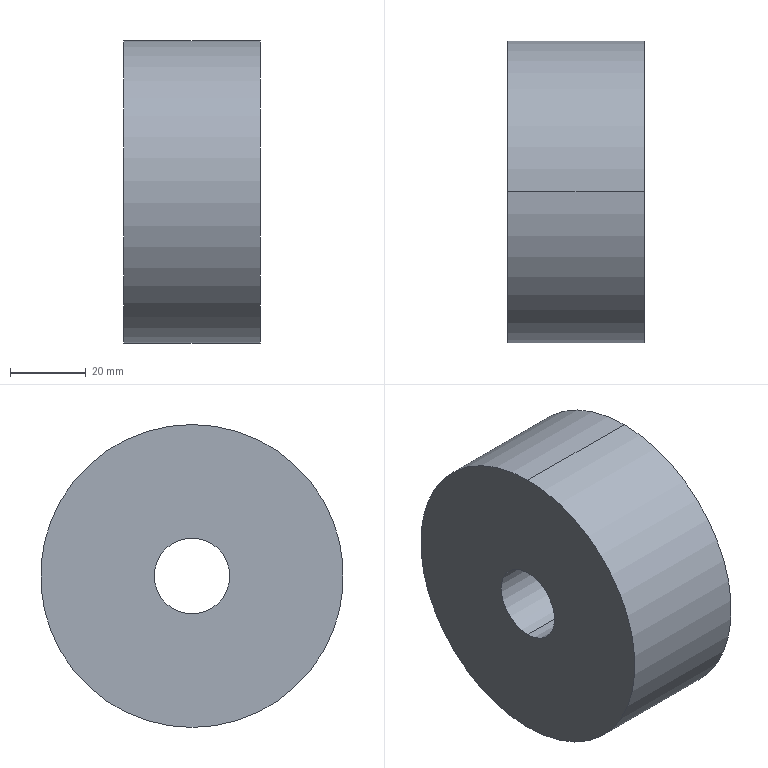Part | SolidWorks | features Revolution 1 | 1 solid | 6 faces | box 36 x 80 x 80 mm | volume 169646 mm3 | cylinder 4 | plane 2 | commonest cylinder face diameters 20 x2 80 x2
STEP:
#1=CARTESIAN_POINT('',(18.,0.,-10.));
#2=VERTEX_POINT('',#1);
#3=CARTESIAN_POINT('',(18.,0.,10.));
#4=VERTEX_POINT('',#3);
#5=CARTESIAN_POINT('',(18.,0.,0.));
#6=DIRECTION('',(-1.,0.,0.));
#7=DIRECTION('',(0.,0.,1.));
#8=AXIS2_PLACEMENT_3D('',#5,#6,#7);
#9=CIRCLE('',#8,10.);
#10=EDGE_CURVE('',#2,#4,#9,.T.);
#11=ORIENTED_EDGE('',*,*,#10,.F.);
#12=CARTESIAN_POINT('',(-18.,0.,-10.));
#13=VERTEX_POINT('',#12);
#14=CARTESIAN_POINT('',(-109.714,0.,-10.));
#15=DIRECTION('',(-1.,0.,0.));
#16=VECTOR('',#15,1000.);
#17=LINE('',#14,#16);
#18=EDGE_CURVE('',#2,#13,#17,.T.);
#19=ORIENTED_EDGE('',*,*,#18,.T.);
#20=CARTESIAN_POINT('',(-18.,0.,10.));
#21=VERTEX_POINT('',#20);
#22=CARTESIAN_POINT('',(-18.,0.,0.));
#23=DIRECTION('',(-1.,0.,0.));
#24=DIRECTION('',(0.,0.,1.));
#25=AXIS2_PLACEMENT_3D('',#22,#23,#24);
#26=CIRCLE('',#25,10.);
#27=EDGE_CURVE('',#13,#21,#26,.T.);
#28=ORIENTED_EDGE('',*,*,#27,.T.);
#29=CARTESIAN_POINT('',(-109.714,0.,10.));
#30=DIRECTION('',(-1.,0.,0.));
#31=VECTOR('',#30,1000.);
#32=LINE('',#29,#31);
#33=EDGE_CURVE('',#4,#21,#32,.T.);
#34=ORIENTED_EDGE('',*,*,#33,.F.);
#35=EDGE_LOOP('',(#11,#19,#28,#34));
#36=FACE_OUTER_BOUND('',#35,.T.);
#37=CARTESIAN_POINT('',(-109.714,0.,0.));
#38=DIRECTION('',(-1.,0.,0.));
#39=DIRECTION('',(0.,0.,1.));
#40=AXIS2_PLACEMENT_3D('',#37,#38,#39);
#41=CYLINDRICAL_SURFACE('',#40,10.);
#42=ADVANCED_FACE('',(#36),#41,.F.);
#43=CARTESIAN_POINT('',(18.,0.,40.));
#44=VERTEX_POINT('',#43);
#45=CARTESIAN_POINT('',(18.,0.,-40.));
#46=VERTEX_POINT('',#45);
#47=CARTESIAN_POINT('',(18.,0.,0.));
#48=DIRECTION('',(-1.,0.,0.));
#49=DIRECTION('',(0.,0.,1.));
#50=AXIS2_PLACEMENT_3D('',#47,#48,#49);
#51=CIRCLE('',#50,40.);
#52=EDGE_CURVE('',#44,#46,#51,.T.);
#53=ORIENTED_EDGE('',*,*,#52,.T.);
#54=CARTESIAN_POINT('',(-18.,0.,-40.));
#55=VERTEX_POINT('',#54);
#56=CARTESIAN_POINT('',(-109.714,0.,-40.));
#57=DIRECTION('',(-1.,0.,0.));
#58=VECTOR('',#57,1000.);
#59=LINE('',#56,#58);
#60=EDGE_CURVE('',#46,#55,#59,.T.);
#61=ORIENTED_EDGE('',*,*,#60,.T.);
#62=CARTESIAN_POINT('',(-18.,0.,40.));
#63=VERTEX_POINT('',#62);
#64=CARTESIAN_POINT('',(-18.,0.,0.));
#65=DIRECTION('',(-1.,0.,0.));
#66=DIRECTION('',(0.,0.,1.));
#67=AXIS2_PLACEMENT_3D('',#64,#65,#66);
#68=CIRCLE('',#67,40.);
#69=EDGE_CURVE('',#63,#55,#68,.T.);
#70=ORIENTED_EDGE('',*,*,#69,.F.);
#71=CARTESIAN_POINT('',(-109.714,0.,40.));
#72=DIRECTION('',(-1.,0.,0.));
#73=VECTOR('',#72,1000.);
#74=LINE('',#71,#73);
#75=EDGE_CURVE('',#44,#63,#74,.T.);
#76=ORIENTED_EDGE('',*,*,#75,.F.);
#77=EDGE_LOOP('',(#53,#61,#70,#76));
#78=FACE_OUTER_BOUND('',#77,.T.);
#79=CARTESIAN_POINT('',(-109.714,0.,0.));
#80=DIRECTION('',(-1.,0.,0.));
#81=DIRECTION('',(0.,0.,1.));
#82=AXIS2_PLACEMENT_3D('',#79,#80,#81);
#83=CYLINDRICAL_SURFACE('',#82,40.);
#84=ADVANCED_FACE('',(#78),#83,.T.);
#85=ORIENTED_EDGE('',*,*,#52,.F.);
#86=CARTESIAN_POINT('',(18.,0.,0.));
#87=DIRECTION('',(-1.,0.,0.));
#88=DIRECTION('',(0.,0.,1.));
#89=AXIS2_PLACEMENT_3D('',#86,#87,#88);
#90=CIRCLE('',#89,40.);
#91=EDGE_CURVE('',#46,#44,#90,.T.);
#92=ORIENTED_EDGE('',*,*,#91,.F.);
#93=EDGE_LOOP('',(#85,#92));
#94=FACE_OUTER_BOUND('',#93,.T.);
#95=CARTESIAN_POINT('',(18.,0.,0.));
#96=DIRECTION('',(-1.,0.,0.));
#97=DIRECTION('',(0.,0.,1.));
#98=AXIS2_PLACEMENT_3D('',#95,#96,#97);
#99=CIRCLE('',#98,10.);
#100=EDGE_CURVE('',#4,#2,#99,.T.);
#101=ORIENTED_EDGE('',*,*,#100,.T.);
#102=ORIENTED_EDGE('',*,*,#10,.T.);
#103=EDGE_LOOP('',(#101,#102));
#104=FACE_BOUND('',#103,.T.);
#105=CARTESIAN_POINT('',(18.,40.,0.));
#106=DIRECTION('',(-1.,0.,0.));
#107=DIRECTION('',(0.,0.,1.));
#108=AXIS2_PLACEMENT_3D('',#105,#106,#107);
#109=PLANE('',#108);
#110=ADVANCED_FACE('',(#94,#104),#109,.F.);
#111=ORIENTED_EDGE('',*,*,#60,.F.);
#112=ORIENTED_EDGE('',*,*,#91,.T.);
#113=ORIENTED_EDGE('',*,*,#75,.T.);
#114=CARTESIAN_POINT('',(-18.,0.,0.));
#115=DIRECTION('',(-1.,0.,0.));
#116=DIRECTION('',(0.,0.,1.));
#117=AXIS2_PLACEMENT_3D('',#114,#115,#116);
#118=CIRCLE('',#117,40.);
#119=EDGE_CURVE('',#55,#63,#118,.T.);
#120=ORIENTED_EDGE('',*,*,#119,.F.);
#121=EDGE_LOOP('',(#111,#112,#113,#120));
#122=FACE_OUTER_BOUND('',#121,.T.);
#123=CARTESIAN_POINT('',(-109.714,0.,0.));
#124=DIRECTION('',(-1.,0.,0.));
#125=DIRECTION('',(0.,0.,1.));
#126=AXIS2_PLACEMENT_3D('',#123,#124,#125);
#127=CYLINDRICAL_SURFACE('',#126,40.);
#128=ADVANCED_FACE('',(#122),#127,.T.);
#129=CARTESIAN_POINT('',(-18.,0.,0.));
#130=DIRECTION('',(-1.,0.,0.));
#131=DIRECTION('',(0.,0.,1.));
#132=AXIS2_PLACEMENT_3D('',#129,#130,#131);
#133=CIRCLE('',#132,10.);
#134=EDGE_CURVE('',#21,#13,#133,.T.);
#135=ORIENTED_EDGE('',*,*,#134,.F.);
#136=ORIENTED_EDGE('',*,*,#27,.F.);
#137=EDGE_LOOP('',(#135,#136));
#138=FACE_BOUND('',#137,.T.);
#139=ORIENTED_EDGE('',*,*,#69,.T.);
#140=ORIENTED_EDGE('',*,*,#119,.T.);
#141=EDGE_LOOP('',(#139,#140));
#142=FACE_OUTER_BOUND('',#141,.T.);
#143=CARTESIAN_POINT('',(-18.,40.,0.));
#144=DIRECTION('',(1.,0.,0.));
#145=DIRECTION('',(0.,0.,-1.));
#146=AXIS2_PLACEMENT_3D('',#143,#144,#145);
#147=PLANE('',#146);
#148=ADVANCED_FACE('',(#138,#142),#147,.F.);
#149=ORIENTED_EDGE('',*,*,#18,.F.);
#150=ORIENTED_EDGE('',*,*,#100,.F.);
#151=ORIENTED_EDGE('',*,*,#33,.T.);
#152=ORIENTED_EDGE('',*,*,#134,.T.);
#153=EDGE_LOOP('',(#149,#150,#151,#152));
#154=FACE_OUTER_BOUND('',#153,.T.);
#155=CARTESIAN_POINT('',(-109.714,0.,0.));
#156=DIRECTION('',(-1.,0.,0.));
#157=DIRECTION('',(0.,0.,1.));
#158=AXIS2_PLACEMENT_3D('',#155,#156,#157);
#159=CYLINDRICAL_SURFACE('',#158,10.);
#160=ADVANCED_FACE('',(#154),#159,.F.);
#161=CLOSED_SHELL('',(#42,#84,#110,#128,#148,#160));
#162=MANIFOLD_SOLID_BREP('',#161);
#163=CARTESIAN_POINT('',(0.,0.,0.));
#164=DIRECTION('',(0.,0.,1.));
#165=DIRECTION('',(1.,0.,0.));
#166=AXIS2_PLACEMENT_3D('',#163,#164,#165);
#167=(LENGTH_UNIT()NAMED_UNIT(*)SI_UNIT(.MILLI.,.METRE.));
#168=UNCERTAINTY_MEASURE_WITH_UNIT(LENGTH_MEASURE(0.00001),#167,'','');
#169=(NAMED_UNIT(*)PLANE_ANGLE_UNIT()SI_UNIT($,.RADIAN.));
#170=(NAMED_UNIT(*)SI_UNIT($,.STERADIAN.)SOLID_ANGLE_UNIT());
#171=(GEOMETRIC_REPRESENTATION_CONTEXT(3)GLOBAL_UNCERTAINTY_ASSIGNED_CONTEXT((#168))GLOBAL_UNIT_ASSIGNED_CONTEXT((#167,#169,#170))REPRESENTATION_CONTEXT('',''));
#172=ADVANCED_BREP_SHAPE_REPRESENTATION('',(#162,#166),#171);